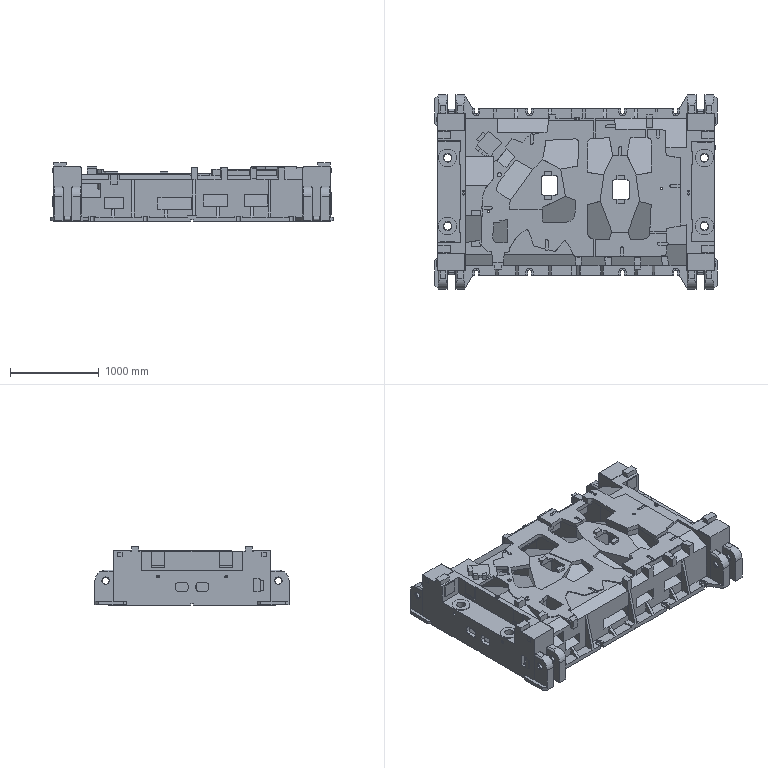Part | NX | features solid 2 | 1 solid | 1873 faces | box 3190 x 2190 x 665 mm | volume 1055357327 mm3 | plane 1346 | cylinder 328 | spline 191 | torus 8 | commonest cylinder face diameters 60 x77 80 x68 83 x48 40 x28 30 x18 32 x18